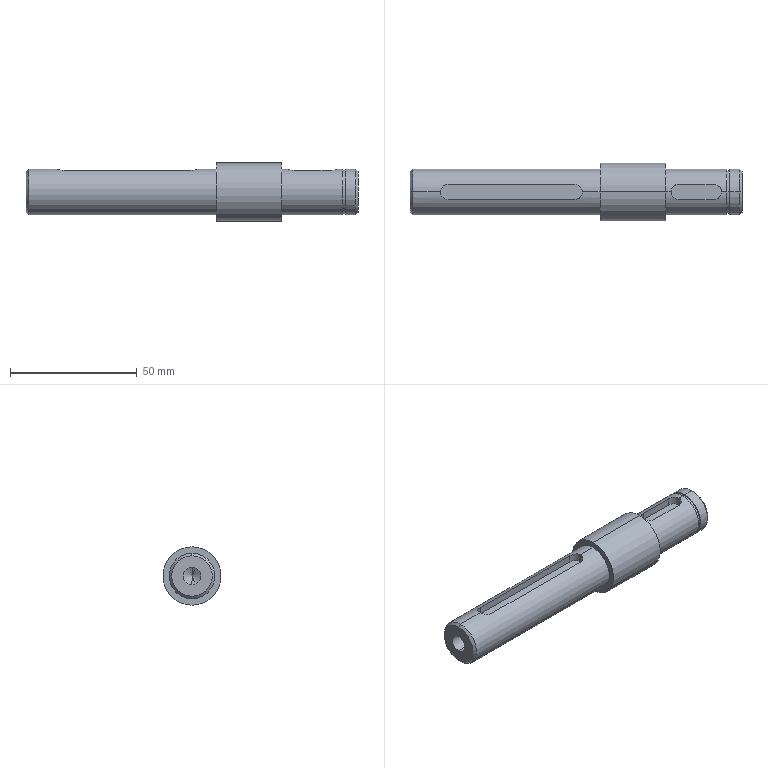Part | STEP file | Reducer shaft | 1 solid | 36 faces | box 131 x 23 x 23 mm | volume 35135 mm3 | cylinder 18 | plane 12 | cone 6 | commonest cylinder face diameters 6 x6 18 x6 6.8 x2 17 x2 23 x2